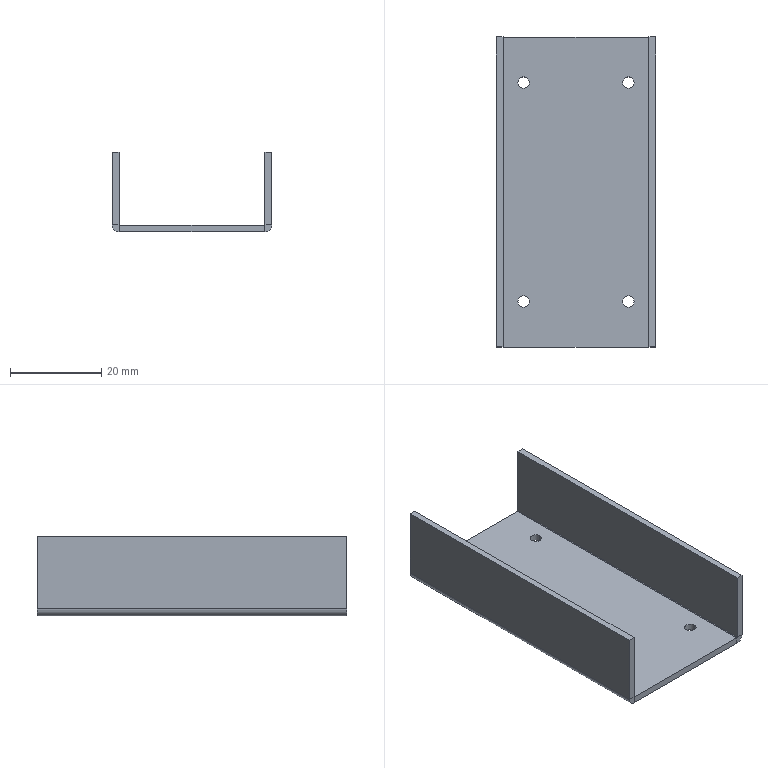Part | 1 solid | 30 faces | box 35 x 68 x 17.5 mm | volume 6730 mm3 | plane 18 | cylinder 12 | commonest cylinder face diameters 2.5 x8 0.2 x2 3.2 x2
STEP:
#1=CARTESIAN_POINT('',(106.15,55.4,-17.5));
#2=VERTEX_POINT('',#1);
#3=CARTESIAN_POINT('',(103.65,55.4,-17.5));
#4=VERTEX_POINT('',#3);
#5=CARTESIAN_POINT('',(104.9,55.4,-17.5));
#6=DIRECTION('',(0.,0.,-1.));
#7=DIRECTION('',(-1.,0.,0.));
#8=AXIS2_PLACEMENT_3D('',#5,#6,#7);
#9=CIRCLE('',#8,1.25);
#10=EDGE_CURVE('',#2,#4,#9,.T.);
#11=ORIENTED_EDGE('',*,*,#10,.F.);
#12=CARTESIAN_POINT('',(106.15,55.4,-19.));
#13=VERTEX_POINT('',#12);
#14=CARTESIAN_POINT('',(106.15,55.4,-1.5));
#15=DIRECTION('',(0.,0.,-1.));
#16=VECTOR('',#15,1000.);
#17=LINE('',#14,#16);
#18=EDGE_CURVE('',#2,#13,#17,.T.);
#19=ORIENTED_EDGE('',*,*,#18,.T.);
#20=CARTESIAN_POINT('',(103.65,55.4,-19.));
#21=VERTEX_POINT('',#20);
#22=CARTESIAN_POINT('',(104.9,55.4,-19.));
#23=DIRECTION('',(0.,0.,-1.));
#24=DIRECTION('',(1.,0.,0.));
#25=AXIS2_PLACEMENT_3D('',#22,#23,#24);
#26=CIRCLE('',#25,1.25);
#27=EDGE_CURVE('',#13,#21,#26,.T.);
#28=ORIENTED_EDGE('',*,*,#27,.T.);
#29=CARTESIAN_POINT('',(103.65,55.4,-1.5));
#30=DIRECTION('',(0.,0.,-1.));
#31=VECTOR('',#30,1000.);
#32=LINE('',#29,#31);
#33=EDGE_CURVE('',#4,#21,#32,.T.);
#34=ORIENTED_EDGE('',*,*,#33,.F.);
#35=EDGE_LOOP('',(#11,#19,#28,#34));
#36=FACE_OUTER_BOUND('',#35,.T.);
#37=CARTESIAN_POINT('',(104.9,55.4,-1.5));
#38=DIRECTION('',(0.,0.,-1.));
#39=DIRECTION('',(-1.,0.,0.));
#40=AXIS2_PLACEMENT_3D('',#37,#38,#39);
#41=CYLINDRICAL_SURFACE('',#40,1.25);
#42=ADVANCED_FACE('',(#36),#41,.F.);
#43=CARTESIAN_POINT('',(83.15,55.4,-17.5));
#44=VERTEX_POINT('',#43);
#45=CARTESIAN_POINT('',(80.65,55.4,-17.5));
#46=VERTEX_POINT('',#45);
#47=CARTESIAN_POINT('',(81.9,55.4,-17.5));
#48=DIRECTION('',(0.,0.,-1.));
#49=DIRECTION('',(-1.,0.,0.));
#50=AXIS2_PLACEMENT_3D('',#47,#48,#49);
#51=CIRCLE('',#50,1.25);
#52=EDGE_CURVE('',#44,#46,#51,.T.);
#53=ORIENTED_EDGE('',*,*,#52,.F.);
#54=CARTESIAN_POINT('',(83.15,55.4,-19.));
#55=VERTEX_POINT('',#54);
#56=CARTESIAN_POINT('',(83.15,55.4,-1.5));
#57=DIRECTION('',(0.,0.,-1.));
#58=VECTOR('',#57,1000.);
#59=LINE('',#56,#58);
#60=EDGE_CURVE('',#44,#55,#59,.T.);
#61=ORIENTED_EDGE('',*,*,#60,.T.);
#62=CARTESIAN_POINT('',(80.65,55.4,-19.));
#63=VERTEX_POINT('',#62);
#64=CARTESIAN_POINT('',(81.9,55.4,-19.));
#65=DIRECTION('',(0.,0.,-1.));
#66=DIRECTION('',(1.,0.,0.));
#67=AXIS2_PLACEMENT_3D('',#64,#65,#66);
#68=CIRCLE('',#67,1.25);
#69=EDGE_CURVE('',#55,#63,#68,.T.);
#70=ORIENTED_EDGE('',*,*,#69,.T.);
#71=CARTESIAN_POINT('',(80.65,55.4,-1.5));
#72=DIRECTION('',(0.,0.,-1.));
#73=VECTOR('',#72,1000.);
#74=LINE('',#71,#73);
#75=EDGE_CURVE('',#46,#63,#74,.T.);
#76=ORIENTED_EDGE('',*,*,#75,.F.);
#77=EDGE_LOOP('',(#53,#61,#70,#76));
#78=FACE_OUTER_BOUND('',#77,.T.);
#79=CARTESIAN_POINT('',(81.9,55.4,-1.5));
#80=DIRECTION('',(0.,0.,-1.));
#81=DIRECTION('',(-1.,0.,0.));
#82=AXIS2_PLACEMENT_3D('',#79,#80,#81);
#83=CYLINDRICAL_SURFACE('',#82,1.25);
#84=ADVANCED_FACE('',(#78),#83,.F.);
#85=CARTESIAN_POINT('',(83.15,103.4,-17.5));
#86=VERTEX_POINT('',#85);
#87=CARTESIAN_POINT('',(80.65,103.4,-17.5));
#88=VERTEX_POINT('',#87);
#89=CARTESIAN_POINT('',(81.9,103.4,-17.5));
#90=DIRECTION('',(0.,0.,-1.));
#91=DIRECTION('',(-1.,0.,0.));
#92=AXIS2_PLACEMENT_3D('',#89,#90,#91);
#93=CIRCLE('',#92,1.25);
#94=EDGE_CURVE('',#86,#88,#93,.T.);
#95=ORIENTED_EDGE('',*,*,#94,.F.);
#96=CARTESIAN_POINT('',(83.15,103.4,-19.));
#97=VERTEX_POINT('',#96);
#98=CARTESIAN_POINT('',(83.15,103.4,-1.5));
#99=DIRECTION('',(0.,0.,-1.));
#100=VECTOR('',#99,1000.);
#101=LINE('',#98,#100);
#102=EDGE_CURVE('',#86,#97,#101,.T.);
#103=ORIENTED_EDGE('',*,*,#102,.T.);
#104=CARTESIAN_POINT('',(80.65,103.4,-19.));
#105=VERTEX_POINT('',#104);
#106=CARTESIAN_POINT('',(81.9,103.4,-19.));
#107=DIRECTION('',(0.,0.,-1.));
#108=DIRECTION('',(1.,0.,0.));
#109=AXIS2_PLACEMENT_3D('',#106,#107,#108);
#110=CIRCLE('',#109,1.25);
#111=EDGE_CURVE('',#97,#105,#110,.T.);
#112=ORIENTED_EDGE('',*,*,#111,.T.);
#113=CARTESIAN_POINT('',(80.65,103.4,-1.5));
#114=DIRECTION('',(0.,0.,-1.));
#115=VECTOR('',#114,1000.);
#116=LINE('',#113,#115);
#117=EDGE_CURVE('',#88,#105,#116,.T.);
#118=ORIENTED_EDGE('',*,*,#117,.F.);
#119=EDGE_LOOP('',(#95,#103,#112,#118));
#120=FACE_OUTER_BOUND('',#119,.T.);
#121=CARTESIAN_POINT('',(81.9,103.4,-1.5));
#122=DIRECTION('',(0.,0.,-1.));
#123=DIRECTION('',(-1.,0.,0.));
#124=AXIS2_PLACEMENT_3D('',#121,#122,#123);
#125=CYLINDRICAL_SURFACE('',#124,1.25);
#126=ADVANCED_FACE('',(#120),#125,.F.);
#127=CARTESIAN_POINT('',(106.15,103.4,-17.5));
#128=VERTEX_POINT('',#127);
#129=CARTESIAN_POINT('',(103.65,103.4,-17.5));
#130=VERTEX_POINT('',#129);
#131=CARTESIAN_POINT('',(104.9,103.4,-17.5));
#132=DIRECTION('',(0.,0.,-1.));
#133=DIRECTION('',(-1.,0.,0.));
#134=AXIS2_PLACEMENT_3D('',#131,#132,#133);
#135=CIRCLE('',#134,1.25);
#136=EDGE_CURVE('',#128,#130,#135,.T.);
#137=ORIENTED_EDGE('',*,*,#136,.F.);
#138=CARTESIAN_POINT('',(106.15,103.4,-19.));
#139=VERTEX_POINT('',#138);
#140=CARTESIAN_POINT('',(106.15,103.4,-1.5));
#141=DIRECTION('',(0.,0.,-1.));
#142=VECTOR('',#141,1000.);
#143=LINE('',#140,#142);
#144=EDGE_CURVE('',#128,#139,#143,.T.);
#145=ORIENTED_EDGE('',*,*,#144,.T.);
#146=CARTESIAN_POINT('',(103.65,103.4,-19.));
#147=VERTEX_POINT('',#146);
#148=CARTESIAN_POINT('',(104.9,103.4,-19.));
#149=DIRECTION('',(0.,0.,-1.));
#150=DIRECTION('',(1.,0.,0.));
#151=AXIS2_PLACEMENT_3D('',#148,#149,#150);
#152=CIRCLE('',#151,1.25);
#153=EDGE_CURVE('',#139,#147,#152,.T.);
#154=ORIENTED_EDGE('',*,*,#153,.T.);
#155=CARTESIAN_POINT('',(103.65,103.4,-1.5));
#156=DIRECTION('',(0.,0.,-1.));
#157=VECTOR('',#156,1000.);
#158=LINE('',#155,#157);
#159=EDGE_CURVE('',#130,#147,#158,.T.);
#160=ORIENTED_EDGE('',*,*,#159,.F.);
#161=EDGE_LOOP('',(#137,#145,#154,#160));
#162=FACE_OUTER_BOUND('',#161,.T.);
#163=CARTESIAN_POINT('',(104.9,103.4,-1.5));
#164=DIRECTION('',(0.,0.,-1.));
#165=DIRECTION('',(-1.,0.,0.));
#166=AXIS2_PLACEMENT_3D('',#163,#164,#165);
#167=CYLINDRICAL_SURFACE('',#166,1.25);
#168=ADVANCED_FACE('',(#162),#167,.F.);
#169=CARTESIAN_POINT('',(75.9,45.4,-1.5));
#170=VERTEX_POINT('',#169);
#171=CARTESIAN_POINT('',(75.9,113.4,-1.5));
#172=VERTEX_POINT('',#171);
#173=CARTESIAN_POINT('',(75.9,113.4,-1.5));
#174=DIRECTION('',(0.,1.,0.));
#175=VECTOR('',#174,1000.);
#176=LINE('',#173,#175);
#177=EDGE_CURVE('',#170,#172,#176,.T.);
#178=ORIENTED_EDGE('',*,*,#177,.F.);
#179=CARTESIAN_POINT('',(77.4,45.4,-1.5));
#180=VERTEX_POINT('',#179);
#181=CARTESIAN_POINT('',(215.568,45.4,-1.5));
#182=DIRECTION('',(-1.,0.,0.));
#183=VECTOR('',#182,1000.);
#184=LINE('',#181,#183);
#185=EDGE_CURVE('',#180,#170,#184,.T.);
#186=ORIENTED_EDGE('',*,*,#185,.F.);
#187=CARTESIAN_POINT('',(77.4,113.4,-1.5));
#188=VERTEX_POINT('',#187);
#189=CARTESIAN_POINT('',(77.4,124.,-1.5));
#190=DIRECTION('',(0.,1.,0.));
#191=VECTOR('',#190,1000.);
#192=LINE('',#189,#191);
#193=EDGE_CURVE('',#180,#188,#192,.T.);
#194=ORIENTED_EDGE('',*,*,#193,.T.);
#195=CARTESIAN_POINT('',(215.568,113.4,-1.5));
#196=DIRECTION('',(-1.,0.,0.));
#197=VECTOR('',#196,1000.);
#198=LINE('',#195,#197);
#199=EDGE_CURVE('',#188,#172,#198,.T.);
#200=ORIENTED_EDGE('',*,*,#199,.T.);
#201=EDGE_LOOP('',(#178,#186,#194,#200));
#202=FACE_OUTER_BOUND('',#201,.T.);
#203=CARTESIAN_POINT('',(215.568,124.,-1.5));
#204=DIRECTION('',(0.,0.,1.));
#205=DIRECTION('',(1.,0.,0.));
#206=AXIS2_PLACEMENT_3D('',#203,#204,#205);
#207=PLANE('',#206);
#208=ADVANCED_FACE('',(#202),#207,.T.);
#209=CARTESIAN_POINT('',(75.9,113.4,-17.4));
#210=VERTEX_POINT('',#209);
#211=CARTESIAN_POINT('',(75.9,113.4,-19.));
#212=DIRECTION('',(0.,0.,1.));
#213=VECTOR('',#212,1000.);
#214=LINE('',#211,#213);
#215=EDGE_CURVE('',#210,#172,#214,.T.);
#216=ORIENTED_EDGE('',*,*,#215,.T.);
#217=ORIENTED_EDGE('',*,*,#199,.F.);
#218=CARTESIAN_POINT('',(77.4,113.4,-17.4));
#219=VERTEX_POINT('',#218);
#220=CARTESIAN_POINT('',(77.4,113.4,-19.));
#221=DIRECTION('',(0.,0.,-1.));
#222=VECTOR('',#221,1000.);
#223=LINE('',#220,#222);
#224=EDGE_CURVE('',#188,#219,#223,.T.);
#225=ORIENTED_EDGE('',*,*,#224,.T.);
#226=CARTESIAN_POINT('',(215.568,113.4,-17.4));
#227=DIRECTION('',(-1.,0.,0.));
#228=VECTOR('',#227,1000.);
#229=LINE('',#226,#228);
#230=EDGE_CURVE('',#219,#210,#229,.T.);
#231=ORIENTED_EDGE('',*,*,#230,.T.);
#232=EDGE_LOOP('',(#216,#217,#225,#231));
#233=FACE_OUTER_BOUND('',#232,.T.);
#234=CARTESIAN_POINT('',(215.568,113.4,-19.));
#235=DIRECTION('',(0.,1.,0.));
#236=DIRECTION('',(1.,0.,0.));
#237=AXIS2_PLACEMENT_3D('',#234,#235,#236);
#238=PLANE('',#237);
#239=ADVANCED_FACE('',(#233),#238,.T.);
#240=ORIENTED_EDGE('',*,*,#215,.F.);
#241=CARTESIAN_POINT('',(75.9,45.4,-17.4));
#242=VERTEX_POINT('',#241);
#243=CARTESIAN_POINT('',(75.9,113.4,-17.4));
#244=DIRECTION('',(0.,-1.,0.));
#245=VECTOR('',#244,1000.);
#246=LINE('',#243,#245);
#247=EDGE_CURVE('',#210,#242,#246,.T.);
#248=ORIENTED_EDGE('',*,*,#247,.T.);
#249=CARTESIAN_POINT('',(75.9,45.4,-19.));
#250=DIRECTION('',(0.,0.,1.));
#251=VECTOR('',#250,1000.);
#252=LINE('',#249,#251);
#253=EDGE_CURVE('',#242,#170,#252,.T.);
#254=ORIENTED_EDGE('',*,*,#253,.T.);
#255=ORIENTED_EDGE('',*,*,#177,.T.);
#256=EDGE_LOOP('',(#240,#248,#254,#255));
#257=FACE_OUTER_BOUND('',#256,.T.);
#258=CARTESIAN_POINT('',(75.9,113.4,-19.));
#259=DIRECTION('',(1.,0.,0.));
#260=DIRECTION('',(0.,1.,0.));
#261=AXIS2_PLACEMENT_3D('',#258,#259,#260);
#262=PLANE('',#261);
#263=ADVANCED_FACE('',(#257),#262,.F.);
#264=ORIENTED_EDGE('',*,*,#253,.F.);
#265=CARTESIAN_POINT('',(77.4,45.4,-17.4));
#266=VERTEX_POINT('',#265);
#267=CARTESIAN_POINT('',(215.568,45.4,-17.4));
#268=DIRECTION('',(-1.,0.,0.));
#269=VECTOR('',#268,1000.);
#270=LINE('',#267,#269);
#271=EDGE_CURVE('',#266,#242,#270,.T.);
#272=ORIENTED_EDGE('',*,*,#271,.F.);
#273=CARTESIAN_POINT('',(77.4,45.4,-19.));
#274=DIRECTION('',(0.,0.,-1.));
#275=VECTOR('',#274,1000.);
#276=LINE('',#273,#275);
#277=EDGE_CURVE('',#180,#266,#276,.T.);
#278=ORIENTED_EDGE('',*,*,#277,.F.);
#279=ORIENTED_EDGE('',*,*,#185,.T.);
#280=EDGE_LOOP('',(#264,#272,#278,#279));
#281=FACE_OUTER_BOUND('',#280,.T.);
#282=CARTESIAN_POINT('',(215.568,45.4,-19.));
#283=DIRECTION('',(0.,-1.,0.));
#284=DIRECTION('',(-1.,0.,0.));
#285=AXIS2_PLACEMENT_3D('',#282,#283,#284);
#286=PLANE('',#285);
#287=ADVANCED_FACE('',(#281),#286,.T.);
#288=ORIENTED_EDGE('',*,*,#277,.T.);
#289=CARTESIAN_POINT('',(77.4,113.4,-17.4));
#290=DIRECTION('',(0.,1.,0.));
#291=VECTOR('',#290,1000.);
#292=LINE('',#289,#291);
#293=EDGE_CURVE('',#266,#219,#292,.T.);
#294=ORIENTED_EDGE('',*,*,#293,.T.);
#295=ORIENTED_EDGE('',*,*,#224,.F.);
#296=ORIENTED_EDGE('',*,*,#193,.F.);
#297=EDGE_LOOP('',(#288,#294,#295,#296));
#298=FACE_OUTER_BOUND('',#297,.T.);
#299=CARTESIAN_POINT('',(77.4,125.5,14.5));
#300=DIRECTION('',(-1.,0.,0.));
#301=DIRECTION('',(0.,0.,1.));
#302=AXIS2_PLACEMENT_3D('',#299,#300,#301);
#303=PLANE('',#302);
#304=ADVANCED_FACE('',(#298),#303,.F.);
#305=CARTESIAN_POINT('',(110.9,113.4,-1.5));
#306=VERTEX_POINT('',#305);
#307=CARTESIAN_POINT('',(110.9,45.4,-1.5));
#308=VERTEX_POINT('',#307);
#309=CARTESIAN_POINT('',(110.9,113.4,-1.5));
#310=DIRECTION('',(0.,-1.,0.));
#311=VECTOR('',#310,1000.);
#312=LINE('',#309,#311);
#313=EDGE_CURVE('',#306,#308,#312,.T.);
#314=ORIENTED_EDGE('',*,*,#313,.F.);
#315=CARTESIAN_POINT('',(109.4,113.4,-1.5));
#316=VERTEX_POINT('',#315);
#317=CARTESIAN_POINT('',(-28.768,113.4,-1.5));
#318=DIRECTION('',(1.,0.,0.));
#319=VECTOR('',#318,1000.);
#320=LINE('',#317,#319);
#321=EDGE_CURVE('',#316,#306,#320,.T.);
#322=ORIENTED_EDGE('',*,*,#321,.F.);
#323=CARTESIAN_POINT('',(109.4,45.4,-1.5));
#324=VERTEX_POINT('',#323);
#325=CARTESIAN_POINT('',(109.4,124.,-1.5));
#326=DIRECTION('',(0.,-1.,0.));
#327=VECTOR('',#326,1000.);
#328=LINE('',#325,#327);
#329=EDGE_CURVE('',#316,#324,#328,.T.);
#330=ORIENTED_EDGE('',*,*,#329,.T.);
#331=CARTESIAN_POINT('',(-28.768,45.4,-1.5));
#332=DIRECTION('',(1.,0.,0.));
#333=VECTOR('',#332,1000.);
#334=LINE('',#331,#333);
#335=EDGE_CURVE('',#324,#308,#334,.T.);
#336=ORIENTED_EDGE('',*,*,#335,.T.);
#337=EDGE_LOOP('',(#314,#322,#330,#336));
#338=FACE_OUTER_BOUND('',#337,.T.);
#339=CARTESIAN_POINT('',(-28.768,124.,-1.5));
#340=DIRECTION('',(0.,0.,1.));
#341=DIRECTION('',(1.,0.,0.));
#342=AXIS2_PLACEMENT_3D('',#339,#340,#341);
#343=PLANE('',#342);
#344=ADVANCED_FACE('',(#338),#343,.T.);
#345=CARTESIAN_POINT('',(110.9,45.4,-17.4));
#346=VERTEX_POINT('',#345);
#347=CARTESIAN_POINT('',(110.9,45.4,-19.));
#348=DIRECTION('',(0.,0.,1.));
#349=VECTOR('',#348,1000.);
#350=LINE('',#347,#349);
#351=EDGE_CURVE('',#346,#308,#350,.T.);
#352=ORIENTED_EDGE('',*,*,#351,.T.);
#353=ORIENTED_EDGE('',*,*,#335,.F.);
#354=CARTESIAN_POINT('',(109.4,45.4,-17.4));
#355=VERTEX_POINT('',#354);
#356=CARTESIAN_POINT('',(109.4,45.4,-19.));
#357=DIRECTION('',(0.,0.,-1.));
#358=VECTOR('',#357,1000.);
#359=LINE('',#356,#358);
#360=EDGE_CURVE('',#324,#355,#359,.T.);
#361=ORIENTED_EDGE('',*,*,#360,.T.);
#362=CARTESIAN_POINT('',(-28.768,45.4,-17.4));
#363=DIRECTION('',(1.,0.,0.));
#364=VECTOR('',#363,1000.);
#365=LINE('',#362,#364);
#366=EDGE_CURVE('',#355,#346,#365,.T.);
#367=ORIENTED_EDGE('',*,*,#366,.T.);
#368=EDGE_LOOP('',(#352,#353,#361,#367));
#369=FACE_OUTER_BOUND('',#368,.T.);
#370=CARTESIAN_POINT('',(-28.768,45.4,-19.));
#371=DIRECTION('',(0.,-1.,0.));
#372=DIRECTION('',(1.,0.,0.));
#373=AXIS2_PLACEMENT_3D('',#370,#371,#372);
#374=PLANE('',#373);
#375=ADVANCED_FACE('',(#369),#374,.T.);
#376=ORIENTED_EDGE('',*,*,#351,.F.);
#377=CARTESIAN_POINT('',(110.9,113.4,-17.4));
#378=VERTEX_POINT('',#377);
#379=CARTESIAN_POINT('',(110.9,45.4,-17.4));
#380=DIRECTION('',(0.,1.,0.));
#381=VECTOR('',#380,1000.);
#382=LINE('',#379,#381);
#383=EDGE_CURVE('',#346,#378,#382,.T.);
#384=ORIENTED_EDGE('',*,*,#383,.T.);
#385=CARTESIAN_POINT('',(110.9,113.4,-19.));
#386=DIRECTION('',(0.,0.,1.));
#387=VECTOR('',#386,1000.);
#388=LINE('',#385,#387);
#389=EDGE_CURVE('',#378,#306,#388,.T.);
#390=ORIENTED_EDGE('',*,*,#389,.T.);
#391=ORIENTED_EDGE('',*,*,#313,.T.);
#392=EDGE_LOOP('',(#376,#384,#390,#391));
#393=FACE_OUTER_BOUND('',#392,.T.);
#394=CARTESIAN_POINT('',(110.9,113.4,-19.));
#395=DIRECTION('',(-1.,0.,0.));
#396=DIRECTION('',(0.,-1.,0.));
#397=AXIS2_PLACEMENT_3D('',#394,#395,#396);
#398=PLANE('',#397);
#399=ADVANCED_FACE('',(#393),#398,.F.);
#400=ORIENTED_EDGE('',*,*,#389,.F.);
#401=CARTESIAN_POINT('',(109.4,113.4,-17.4));
#402=VERTEX_POINT('',#401);
#403=CARTESIAN_POINT('',(-28.768,113.4,-17.4));
#404=DIRECTION('',(1.,0.,0.));
#405=VECTOR('',#404,1000.);
#406=LINE('',#403,#405);
#407=EDGE_CURVE('',#402,#378,#406,.T.);
#408=ORIENTED_EDGE('',*,*,#407,.F.);
#409=CARTESIAN_POINT('',(109.4,113.4,-19.));
#410=DIRECTION('',(0.,0.,-1.));
#411=VECTOR('',#410,1000.);
#412=LINE('',#409,#411);
#413=EDGE_CURVE('',#316,#402,#412,.T.);
#414=ORIENTED_EDGE('',*,*,#413,.F.);
#415=ORIENTED_EDGE('',*,*,#321,.T.);
#416=EDGE_LOOP('',(#400,#408,#414,#415));
#417=FACE_OUTER_BOUND('',#416,.T.);
#418=CARTESIAN_POINT('',(-28.768,113.4,-19.));
#419=DIRECTION('',(0.,1.,0.));
#420=DIRECTION('',(-1.,0.,0.));
#421=AXIS2_PLACEMENT_3D('',#418,#419,#420);
#422=PLANE('',#421);
#423=ADVANCED_FACE('',(#417),#422,.T.);
#424=ORIENTED_EDGE('',*,*,#413,.T.);
#425=CARTESIAN_POINT('',(109.4,45.4,-17.4));
#426=DIRECTION('',(0.,-1.,0.));
#427=VECTOR('',#426,1000.);
#428=LINE('',#425,#427);
#429=EDGE_CURVE('',#402,#355,#428,.T.);
#430=ORIENTED_EDGE('',*,*,#429,.T.);
#431=ORIENTED_EDGE('',*,*,#360,.F.);
#432=ORIENTED_EDGE('',*,*,#329,.F.);
#433=EDGE_LOOP('',(#424,#430,#431,#432));
#434=FACE_OUTER_BOUND('',#433,.T.);
#435=CARTESIAN_POINT('',(109.4,125.5,14.5));
#436=DIRECTION('',(1.,0.,0.));
#437=DIRECTION('',(0.,0.,-1.));
#438=AXIS2_PLACEMENT_3D('',#435,#436,#437);
#439=PLANE('',#438);
#440=ADVANCED_FACE('',(#434),#439,.F.);
#441=CARTESIAN_POINT('',(104.9,55.4,-19.));
#442=DIRECTION('',(0.,0.,-1.));
#443=DIRECTION('',(1.,0.,0.));
#444=AXIS2_PLACEMENT_3D('',#441,#442,#443);
#445=CIRCLE('',#444,1.25);
#446=EDGE_CURVE('',#21,#13,#445,.T.);
#447=ORIENTED_EDGE('',*,*,#446,.F.);
#448=ORIENTED_EDGE('',*,*,#27,.F.);
#449=EDGE_LOOP('',(#447,#448));
#450=FACE_BOUND('',#449,.T.);
#451=CARTESIAN_POINT('',(81.9,55.4,-19.));
#452=DIRECTION('',(0.,0.,-1.));
#453=DIRECTION('',(1.,0.,0.));
#454=AXIS2_PLACEMENT_3D('',#451,#452,#453);
#455=CIRCLE('',#454,1.25);
#456=EDGE_CURVE('',#63,#55,#455,.T.);
#457=ORIENTED_EDGE('',*,*,#456,.F.);
#458=ORIENTED_EDGE('',*,*,#69,.F.);
#459=EDGE_LOOP('',(#457,#458));
#460=FACE_BOUND('',#459,.T.);
#461=CARTESIAN_POINT('',(81.9,103.4,-19.));
#462=DIRECTION('',(0.,0.,-1.));
#463=DIRECTION('',(1.,0.,0.));
#464=AXIS2_PLACEMENT_3D('',#461,#462,#463);
#465=CIRCLE('',#464,1.25);
#466=EDGE_CURVE('',#105,#97,#465,.T.);
#467=ORIENTED_EDGE('',*,*,#466,.F.);
#468=ORIENTED_EDGE('',*,*,#111,.F.);
#469=EDGE_LOOP('',(#467,#468));
#470=FACE_BOUND('',#469,.T.);
#471=CARTESIAN_POINT('',(104.9,103.4,-19.));
#472=DIRECTION('',(0.,0.,-1.));
#473=DIRECTION('',(1.,0.,0.));
#474=AXIS2_PLACEMENT_3D('',#471,#472,#473);
#475=CIRCLE('',#474,1.25);
#476=EDGE_CURVE('',#147,#139,#475,.T.);
#477=ORIENTED_EDGE('',*,*,#476,.F.);
#478=ORIENTED_EDGE('',*,*,#153,.F.);
#479=EDGE_LOOP('',(#477,#478));
#480=FACE_BOUND('',#479,.T.);
#481=CARTESIAN_POINT('',(77.5,113.4,-19.));
#482=VERTEX_POINT('',#481);
#483=CARTESIAN_POINT('',(77.5,45.4,-19.));
#484=VERTEX_POINT('',#483);
#485=CARTESIAN_POINT('',(77.5,113.4,-19.));
#486=DIRECTION('',(0.,-1.,0.));
#487=VECTOR('',#486,1000.);
#488=LINE('',#485,#487);
#489=EDGE_CURVE('',#482,#484,#488,.T.);
#490=ORIENTED_EDGE('',*,*,#489,.F.);
#491=CARTESIAN_POINT('',(109.3,113.4,-19.));
#492=VERTEX_POINT('',#491);
#493=CARTESIAN_POINT('',(110.9,113.4,-19.));
#494=DIRECTION('',(1.,0.,0.));
#495=VECTOR('',#494,1000.);
#496=LINE('',#493,#495);
#497=EDGE_CURVE('',#482,#492,#496,.T.);
#498=ORIENTED_EDGE('',*,*,#497,.T.);
#499=CARTESIAN_POINT('',(109.3,45.4,-19.));
#500=VERTEX_POINT('',#499);
#501=CARTESIAN_POINT('',(109.3,45.4,-19.));
#502=DIRECTION('',(0.,1.,0.));
#503=VECTOR('',#502,1000.);
#504=LINE('',#501,#503);
#505=EDGE_CURVE('',#500,#492,#504,.T.);
#506=ORIENTED_EDGE('',*,*,#505,.F.);
#507=CARTESIAN_POINT('',(110.9,45.4,-19.));
#508=DIRECTION('',(-1.,0.,0.));
#509=VECTOR('',#508,1000.);
#510=LINE('',#507,#509);
#511=EDGE_CURVE('',#500,#484,#510,.T.);
#512=ORIENTED_EDGE('',*,*,#511,.T.);
#513=EDGE_LOOP('',(#490,#498,#506,#512));
#514=FACE_OUTER_BOUND('',#513,.T.);
#515=CARTESIAN_POINT('',(0.,0.,-19.));
#516=DIRECTION('',(0.,0.,1.));
#517=DIRECTION('',(1.,0.,0.));
#518=AXIS2_PLACEMENT_3D('',#515,#516,#517);
#519=PLANE('',#518);
#520=ADVANCED_FACE('',(#450,#460,#470,#480,#514),#519,.F.);
#521=CARTESIAN_POINT('',(104.9,55.4,-17.5));
#522=DIRECTION('',(0.,0.,-1.));
#523=DIRECTION('',(-1.,0.,0.));
#524=AXIS2_PLACEMENT_3D('',#521,#522,#523);
#525=CIRCLE('',#524,1.25);
#526=EDGE_CURVE('',#4,#2,#525,.T.);
#527=ORIENTED_EDGE('',*,*,#526,.T.);
#528=ORIENTED_EDGE('',*,*,#10,.T.);
#529=EDGE_LOOP('',(#527,#528));
#530=FACE_BOUND('',#529,.T.);
#531=CARTESIAN_POINT('',(81.9,55.4,-17.5));
#532=DIRECTION('',(0.,0.,-1.));
#533=DIRECTION('',(-1.,0.,0.));
#534=AXIS2_PLACEMENT_3D('',#531,#532,#533);
#535=CIRCLE('',#534,1.25);
#536=EDGE_CURVE('',#46,#44,#535,.T.);
#537=ORIENTED_EDGE('',*,*,#536,.T.);
#538=ORIENTED_EDGE('',*,*,#52,.T.);
#539=EDGE_LOOP('',(#537,#538));
#540=FACE_BOUND('',#539,.T.);
#541=CARTESIAN_POINT('',(81.9,103.4,-17.5));
#542=DIRECTION('',(0.,0.,-1.));
#543=DIRECTION('',(-1.,0.,0.));
#544=AXIS2_PLACEMENT_3D('',#541,#542,#543);
#545=CIRCLE('',#544,1.25);
#546=EDGE_CURVE('',#88,#86,#545,.T.);
#547=ORIENTED_EDGE('',*,*,#546,.T.);
#548=ORIENTED_EDGE('',*,*,#94,.T.);
#549=EDGE_LOOP('',(#547,#548));
#550=FACE_BOUND('',#549,.T.);
#551=CARTESIAN_POINT('',(104.9,103.4,-17.5));
#552=DIRECTION('',(0.,0.,-1.));
#553=DIRECTION('',(-1.,0.,0.));
#554=AXIS2_PLACEMENT_3D('',#551,#552,#553);
#555=CIRCLE('',#554,1.25);
#556=EDGE_CURVE('',#130,#128,#555,.T.);
#557=ORIENTED_EDGE('',*,*,#556,.T.);
#558=ORIENTED_EDGE('',*,*,#136,.T.);
#559=EDGE_LOOP('',(#557,#558));
#560=FACE_BOUND('',#559,.T.);
#561=CARTESIAN_POINT('',(77.5,45.4,-17.5));
#562=VERTEX_POINT('',#561);
#563=CARTESIAN_POINT('',(77.5,113.4,-17.5));
#564=VERTEX_POINT('',#563);
#565=CARTESIAN_POINT('',(77.5,113.4,-17.5));
#566=DIRECTION('',(0.,1.,0.));
#567=VECTOR('',#566,1000.);
#568=LINE('',#565,#567);
#569=EDGE_CURVE('',#562,#564,#568,.T.);
#570=ORIENTED_EDGE('',*,*,#569,.F.);
#571=CARTESIAN_POINT('',(109.3,45.4,-17.5));
#572=VERTEX_POINT('',#571);
#573=CARTESIAN_POINT('',(110.9,45.4,-17.5));
#574=DIRECTION('',(-1.,0.,0.));
#575=VECTOR('',#574,1000.);
#576=LINE('',#573,#575);
#577=EDGE_CURVE('',#572,#562,#576,.T.);
#578=ORIENTED_EDGE('',*,*,#577,.F.);
#579=CARTESIAN_POINT('',(109.3,113.4,-17.5));
#580=VERTEX_POINT('',#579);
#581=CARTESIAN_POINT('',(109.3,45.4,-17.5));
#582=DIRECTION('',(0.,-1.,0.));
#583=VECTOR('',#582,1000.);
#584=LINE('',#581,#583);
#585=EDGE_CURVE('',#580,#572,#584,.T.);
#586=ORIENTED_EDGE('',*,*,#585,.F.);
#587=CARTESIAN_POINT('',(110.9,113.4,-17.5));
#588=DIRECTION('',(1.,0.,0.));
#589=VECTOR('',#588,1000.);
#590=LINE('',#587,#589);
#591=EDGE_CURVE('',#564,#580,#590,.T.);
#592=ORIENTED_EDGE('',*,*,#591,.F.);
#593=EDGE_LOOP('',(#570,#578,#586,#592));
#594=FACE_OUTER_BOUND('',#593,.T.);
#595=CARTESIAN_POINT('',(77.4,125.5,-17.5));
#596=DIRECTION('',(0.,0.,-1.));
#597=DIRECTION('',(-1.,0.,0.));
#598=AXIS2_PLACEMENT_3D('',#595,#596,#597);
#599=PLANE('',#598);
#600=ADVANCED_FACE('',(#530,#540,#550,#560,#594),#599,.F.);
#601=ORIENTED_EDGE('',*,*,#144,.F.);
#602=ORIENTED_EDGE('',*,*,#556,.F.);
#603=ORIENTED_EDGE('',*,*,#159,.T.);
#604=ORIENTED_EDGE('',*,*,#476,.T.);
#605=EDGE_LOOP('',(#601,#602,#603,#604));
#606=FACE_OUTER_BOUND('',#605,.T.);
#607=CARTESIAN_POINT('',(104.9,103.4,-1.5));
#608=DIRECTION('',(0.,0.,-1.));
#609=DIRECTION('',(-1.,0.,0.));
#610=AXIS2_PLACEMENT_3D('',#607,#608,#609);
#611=CYLINDRICAL_SURFACE('',#610,1.25);
#612=ADVANCED_FACE('',(#606),#611,.F.);
#613=ORIENTED_EDGE('',*,*,#102,.F.);
#614=ORIENTED_EDGE('',*,*,#546,.F.);
#615=ORIENTED_EDGE('',*,*,#117,.T.);
#616=ORIENTED_EDGE('',*,*,#466,.T.);
#617=EDGE_LOOP('',(#613,#614,#615,#616));
#618=FACE_OUTER_BOUND('',#617,.T.);
#619=CARTESIAN_POINT('',(81.9,103.4,-1.5));
#620=DIRECTION('',(0.,0.,-1.));
#621=DIRECTION('',(-1.,0.,0.));
#622=AXIS2_PLACEMENT_3D('',#619,#620,#621);
#623=CYLINDRICAL_SURFACE('',#622,1.25);
#624=ADVANCED_FACE('',(#618),#623,.F.);
#625=ORIENTED_EDGE('',*,*,#60,.F.);
#626=ORIENTED_EDGE('',*,*,#536,.F.);
#627=ORIENTED_EDGE('',*,*,#75,.T.);
#628=ORIENTED_EDGE('',*,*,#456,.T.);
#629=EDGE_LOOP('',(#625,#626,#627,#628));
#630=FACE_OUTER_BOUND('',#629,.T.);
#631=CARTESIAN_POINT('',(81.9,55.4,-1.5));
#632=DIRECTION('',(0.,0.,-1.));
#633=DIRECTION('',(-1.,0.,0.));
#634=AXIS2_PLACEMENT_3D('',#631,#632,#633);
#635=CYLINDRICAL_SURFACE('',#634,1.25);
#636=ADVANCED_FACE('',(#630),#635,.F.);
#637=ORIENTED_EDGE('',*,*,#18,.F.);
#638=ORIENTED_EDGE('',*,*,#526,.F.);
#639=ORIENTED_EDGE('',*,*,#33,.T.);
#640=ORIENTED_EDGE('',*,*,#446,.T.);
#641=EDGE_LOOP('',(#637,#638,#639,#640));
#642=FACE_OUTER_BOUND('',#641,.T.);
#643=CARTESIAN_POINT('',(104.9,55.4,-1.5));
#644=DIRECTION('',(0.,0.,-1.));
#645=DIRECTION('',(-1.,0.,0.));
#646=AXIS2_PLACEMENT_3D('',#643,#644,#645);
#647=CYLINDRICAL_SURFACE('',#646,1.25);
#648=ADVANCED_FACE('',(#642),#647,.F.);
#649=ORIENTED_EDGE('',*,*,#497,.F.);
#650=CARTESIAN_POINT('',(77.5,113.4,131.136));
#651=DIRECTION('',(0.,0.,-1.));
#652=VECTOR('',#651,1000.);
#653=LINE('',#650,#652);
#654=EDGE_CURVE('',#564,#482,#653,.T.);
#655=ORIENTED_EDGE('',*,*,#654,.F.);
#656=ORIENTED_EDGE('',*,*,#591,.T.);
#657=CARTESIAN_POINT('',(109.3,113.4,131.136));
#658=DIRECTION('',(0.,0.,-1.));
#659=VECTOR('',#658,1000.);
#660=LINE('',#657,#659);
#661=EDGE_CURVE('',#580,#492,#660,.T.);
#662=ORIENTED_EDGE('',*,*,#661,.T.);
#663=EDGE_LOOP('',(#649,#655,#656,#662));
#664=FACE_OUTER_BOUND('',#663,.T.);
#665=CARTESIAN_POINT('',(110.9,113.4,131.136));
#666=DIRECTION('',(0.,1.,0.));
#667=DIRECTION('',(-1.,0.,0.));
#668=AXIS2_PLACEMENT_3D('',#665,#666,#667);
#669=PLANE('',#668);
#670=ADVANCED_FACE('',(#664),#669,.T.);
#671=ORIENTED_EDGE('',*,*,#511,.F.);
#672=CARTESIAN_POINT('',(109.3,45.4,131.136));
#673=DIRECTION('',(0.,0.,-1.));
#674=VECTOR('',#673,1000.);
#675=LINE('',#672,#674);
#676=EDGE_CURVE('',#572,#500,#675,.T.);
#677=ORIENTED_EDGE('',*,*,#676,.F.);
#678=ORIENTED_EDGE('',*,*,#577,.T.);
#679=CARTESIAN_POINT('',(77.5,45.4,131.136));
#680=DIRECTION('',(0.,0.,-1.));
#681=VECTOR('',#680,1000.);
#682=LINE('',#679,#681);
#683=EDGE_CURVE('',#562,#484,#682,.T.);
#684=ORIENTED_EDGE('',*,*,#683,.T.);
#685=EDGE_LOOP('',(#671,#677,#678,#684));
#686=FACE_OUTER_BOUND('',#685,.T.);
#687=CARTESIAN_POINT('',(110.9,45.4,131.136));
#688=DIRECTION('',(0.,-1.,0.));
#689=DIRECTION('',(1.,0.,0.));
#690=AXIS2_PLACEMENT_3D('',#687,#688,#689);
#691=PLANE('',#690);
#692=ADVANCED_FACE('',(#686),#691,.T.);
#693=ORIENTED_EDGE('',*,*,#366,.F.);
#694=CARTESIAN_POINT('',(109.3,45.4,-17.4));
#695=DIRECTION('',(0.,1.,0.));
#696=DIRECTION('',(0.,0.,1.));
#697=AXIS2_PLACEMENT_3D('',#694,#695,#696);
#698=CIRCLE('',#697,0.1);
#699=EDGE_CURVE('',#355,#572,#698,.T.);
#700=ORIENTED_EDGE('',*,*,#699,.T.);
#701=ORIENTED_EDGE('',*,*,#676,.T.);
#702=CARTESIAN_POINT('',(109.3,45.4,-17.4));
#703=DIRECTION('',(0.,1.,0.));
#704=DIRECTION('',(0.,0.,1.));
#705=AXIS2_PLACEMENT_3D('',#702,#703,#704);
#706=CIRCLE('',#705,1.6);
#707=EDGE_CURVE('',#346,#500,#706,.T.);
#708=ORIENTED_EDGE('',*,*,#707,.F.);
#709=EDGE_LOOP('',(#693,#700,#701,#708));
#710=FACE_OUTER_BOUND('',#709,.T.);
#711=CARTESIAN_POINT('',(109.3,45.4,-17.4));
#712=DIRECTION('',(0.,-1.,0.));
#713=DIRECTION('',(0.,0.,-1.));
#714=AXIS2_PLACEMENT_3D('',#711,#712,#713);
#715=PLANE('',#714);
#716=ADVANCED_FACE('',(#710),#715,.T.);
#717=CARTESIAN_POINT('',(109.3,113.4,-17.4));
#718=DIRECTION('',(0.,-1.,0.));
#719=DIRECTION('',(0.,0.,1.));
#720=AXIS2_PLACEMENT_3D('',#717,#718,#719);
#721=CIRCLE('',#720,0.1);
#722=EDGE_CURVE('',#580,#402,#721,.T.);
#723=ORIENTED_EDGE('',*,*,#722,.T.);
#724=ORIENTED_EDGE('',*,*,#407,.T.);
#725=CARTESIAN_POINT('',(109.3,113.4,-17.4));
#726=DIRECTION('',(0.,-1.,0.));
#727=DIRECTION('',(0.,0.,1.));
#728=AXIS2_PLACEMENT_3D('',#725,#726,#727);
#729=CIRCLE('',#728,1.6);
#730=EDGE_CURVE('',#492,#378,#729,.T.);
#731=ORIENTED_EDGE('',*,*,#730,.F.);
#732=ORIENTED_EDGE('',*,*,#661,.F.);
#733=EDGE_LOOP('',(#723,#724,#731,#732));
#734=FACE_OUTER_BOUND('',#733,.T.);
#735=CARTESIAN_POINT('',(109.3,113.4,-17.4));
#736=DIRECTION('',(0.,1.,0.));
#737=DIRECTION('',(0.,0.,1.));
#738=AXIS2_PLACEMENT_3D('',#735,#736,#737);
#739=PLANE('',#738);
#740=ADVANCED_FACE('',(#734),#739,.T.);
#741=ORIENTED_EDGE('',*,*,#505,.T.);
#742=ORIENTED_EDGE('',*,*,#730,.T.);
#743=ORIENTED_EDGE('',*,*,#383,.F.);
#744=ORIENTED_EDGE('',*,*,#707,.T.);
#745=EDGE_LOOP('',(#741,#742,#743,#744));
#746=FACE_OUTER_BOUND('',#745,.T.);
#747=CARTESIAN_POINT('',(109.3,-48.819,-17.4));
#748=DIRECTION('',(0.,1.,0.));
#749=DIRECTION('',(0.,0.,1.));
#750=AXIS2_PLACEMENT_3D('',#747,#748,#749);
#751=CYLINDRICAL_SURFACE('',#750,1.6);
#752=ADVANCED_FACE('',(#746),#751,.T.);
#753=ORIENTED_EDGE('',*,*,#585,.T.);
#754=ORIENTED_EDGE('',*,*,#699,.F.);
#755=ORIENTED_EDGE('',*,*,#429,.F.);
#756=ORIENTED_EDGE('',*,*,#722,.F.);
#757=EDGE_LOOP('',(#753,#754,#755,#756));
#758=FACE_OUTER_BOUND('',#757,.T.);
#759=CARTESIAN_POINT('',(109.3,-48.819,-17.4));
#760=DIRECTION('',(0.,1.,0.));
#761=DIRECTION('',(0.,0.,1.));
#762=AXIS2_PLACEMENT_3D('',#759,#760,#761);
#763=CYLINDRICAL_SURFACE('',#762,0.1);
#764=ADVANCED_FACE('',(#758),#763,.F.);
#765=ORIENTED_EDGE('',*,*,#230,.F.);
#766=CARTESIAN_POINT('',(77.5,113.4,-17.4));
#767=DIRECTION('',(0.,-1.,0.));
#768=DIRECTION('',(0.,0.,-1.));
#769=AXIS2_PLACEMENT_3D('',#766,#767,#768);
#770=CIRCLE('',#769,0.1);
#771=EDGE_CURVE('',#219,#564,#770,.T.);
#772=ORIENTED_EDGE('',*,*,#771,.T.);
#773=ORIENTED_EDGE('',*,*,#654,.T.);
#774=CARTESIAN_POINT('',(77.5,113.4,-17.4));
#775=DIRECTION('',(0.,-1.,0.));
#776=DIRECTION('',(0.,0.,-1.));
#777=AXIS2_PLACEMENT_3D('',#774,#775,#776);
#778=CIRCLE('',#777,1.6);
#779=EDGE_CURVE('',#210,#482,#778,.T.);
#780=ORIENTED_EDGE('',*,*,#779,.F.);
#781=EDGE_LOOP('',(#765,#772,#773,#780));
#782=FACE_OUTER_BOUND('',#781,.T.);
#783=CARTESIAN_POINT('',(77.5,113.4,-17.4));
#784=DIRECTION('',(0.,1.,0.));
#785=DIRECTION('',(0.,0.,1.));
#786=AXIS2_PLACEMENT_3D('',#783,#784,#785);
#787=PLANE('',#786);
#788=ADVANCED_FACE('',(#782),#787,.T.);
#789=CARTESIAN_POINT('',(77.5,45.4,-17.4));
#790=DIRECTION('',(0.,1.,0.));
#791=DIRECTION('',(0.,0.,-1.));
#792=AXIS2_PLACEMENT_3D('',#789,#790,#791);
#793=CIRCLE('',#792,0.1);
#794=EDGE_CURVE('',#562,#266,#793,.T.);
#795=ORIENTED_EDGE('',*,*,#794,.T.);
#796=ORIENTED_EDGE('',*,*,#271,.T.);
#797=CARTESIAN_POINT('',(77.5,45.4,-17.4));
#798=DIRECTION('',(0.,1.,0.));
#799=DIRECTION('',(0.,0.,-1.));
#800=AXIS2_PLACEMENT_3D('',#797,#798,#799);
#801=CIRCLE('',#800,1.6);
#802=EDGE_CURVE('',#484,#242,#801,.T.);
#803=ORIENTED_EDGE('',*,*,#802,.F.);
#804=ORIENTED_EDGE('',*,*,#683,.F.);
#805=EDGE_LOOP('',(#795,#796,#803,#804));
#806=FACE_OUTER_BOUND('',#805,.T.);
#807=CARTESIAN_POINT('',(77.5,45.4,-17.4));
#808=DIRECTION('',(0.,-1.,0.));
#809=DIRECTION('',(0.,0.,-1.));
#810=AXIS2_PLACEMENT_3D('',#807,#808,#809);
#811=PLANE('',#810);
#812=ADVANCED_FACE('',(#806),#811,.T.);
#813=ORIENTED_EDGE('',*,*,#489,.T.);
#814=ORIENTED_EDGE('',*,*,#802,.T.);
#815=ORIENTED_EDGE('',*,*,#247,.F.);
#816=ORIENTED_EDGE('',*,*,#779,.T.);
#817=EDGE_LOOP('',(#813,#814,#815,#816));
#818=FACE_OUTER_BOUND('',#817,.T.);
#819=CARTESIAN_POINT('',(77.5,199.657,-17.4));
#820=DIRECTION('',(0.,-1.,0.));
#821=DIRECTION('',(0.,0.,-1.));
#822=AXIS2_PLACEMENT_3D('',#819,#820,#821);
#823=CYLINDRICAL_SURFACE('',#822,1.6);
#824=ADVANCED_FACE('',(#818),#823,.T.);
#825=ORIENTED_EDGE('',*,*,#569,.T.);
#826=ORIENTED_EDGE('',*,*,#771,.F.);
#827=ORIENTED_EDGE('',*,*,#293,.F.);
#828=ORIENTED_EDGE('',*,*,#794,.F.);
#829=EDGE_LOOP('',(#825,#826,#827,#828));
#830=FACE_OUTER_BOUND('',#829,.T.);
#831=CARTESIAN_POINT('',(77.5,199.657,-17.4));
#832=DIRECTION('',(0.,-1.,0.));
#833=DIRECTION('',(0.,0.,-1.));
#834=AXIS2_PLACEMENT_3D('',#831,#832,#833);
#835=CYLINDRICAL_SURFACE('',#834,0.1);
#836=ADVANCED_FACE('',(#830),#835,.F.);
#837=CLOSED_SHELL('',(#42,#84,#126,#168,#208,#239,#263,#287,#304,#344,#375,#399,#423,#440,#520,#600,#612,#624,#636,#648,#670,#692,#716,#740,#752,#764,#788,#812,#824,#836));
#838=MANIFOLD_SOLID_BREP('',#837);
#839=CARTESIAN_POINT('',(0.,0.,0.));
#840=DIRECTION('',(0.,0.,1.));
#841=DIRECTION('',(1.,0.,0.));
#842=AXIS2_PLACEMENT_3D('',#839,#840,#841);
#843=(LENGTH_UNIT()NAMED_UNIT(*)SI_UNIT(.MILLI.,.METRE.));
#844=UNCERTAINTY_MEASURE_WITH_UNIT(LENGTH_MEASURE(0.00001),#843,'','');
#845=(NAMED_UNIT(*)PLANE_ANGLE_UNIT()SI_UNIT($,.RADIAN.));
#846=(NAMED_UNIT(*)SI_UNIT($,.STERADIAN.)SOLID_ANGLE_UNIT());
#847=(GEOMETRIC_REPRESENTATION_CONTEXT(3)GLOBAL_UNCERTAINTY_ASSIGNED_CONTEXT((#844))GLOBAL_UNIT_ASSIGNED_CONTEXT((#843,#845,#846))REPRESENTATION_CONTEXT('',''));
#848=ADVANCED_BREP_SHAPE_REPRESENTATION('',(#838,#842),#847);